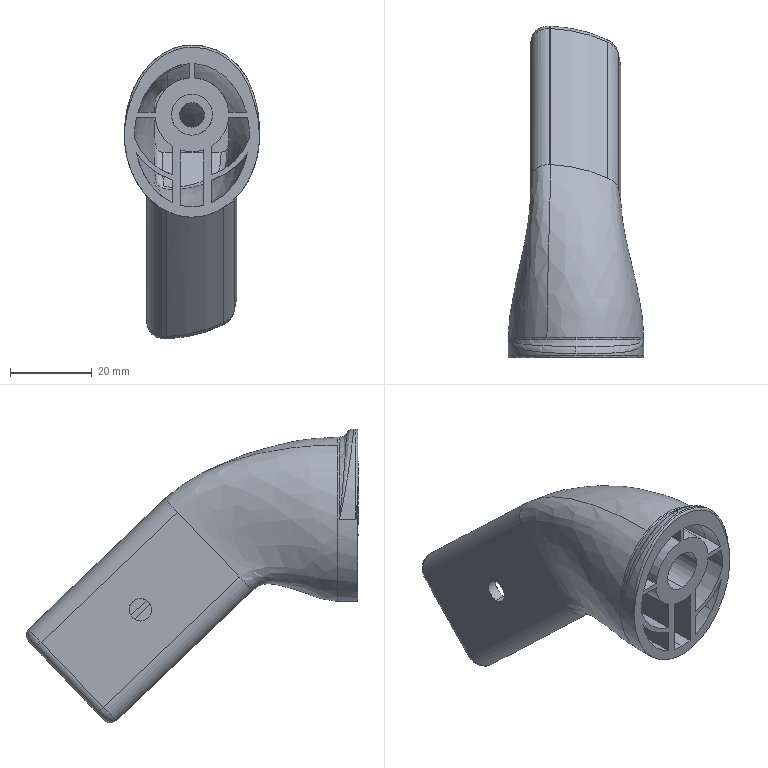Part | SolidWorks | features BaseBody 1 | 1 solid | 161 faces | box 33 x 80.996 x 71.706 mm | volume 27661 mm3 | plane 49 | spline 46 | cylinder 45 | torus 21 | commonest cylinder face diameters 4 x6 18 x6 6 x5 2 x3 9 x3 5.5 x2